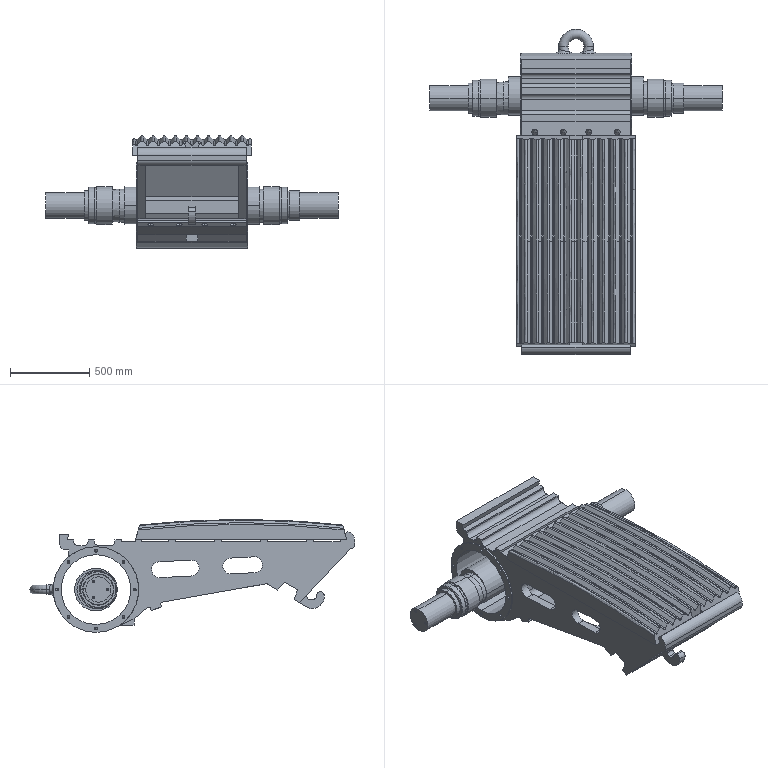Part | SolidWorks | features CompositeCurve 1 | 6 solids | 582 faces | box 1846 x 2050 x 710.858 mm | volume 325009272 mm3 | plane 217 | cylinder 202 | cone 97 | torus 62 | spline 4 | commonest cylinder face diameters 17.5 x40 100 x19 140 x18 36 x16 14 x12 240 x10